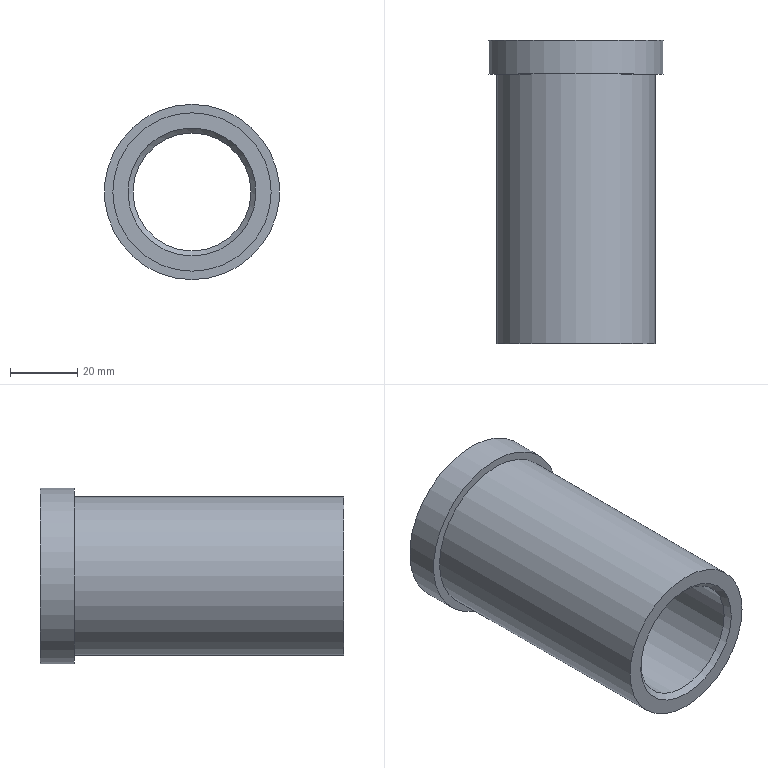Part | STEP file | GUIDE2_id254_x_t | 1 solid | 8 faces | box 52 x 90 x 52 mm | volume 73227 mm3 | cylinder 3 | plane 3 | cone 2 | commonest cylinder face diameters 35 x1 47 x1 52 x1
STEP:
#1=CARTESIAN_POINT('',(-162.,90.5,-216.25));
#2=VERTEX_POINT('',#1);
#3=CARTESIAN_POINT('',(-162.,90.5,-235.));
#4=DIRECTION('',(0.,1.,0.));
#5=DIRECTION('',(0.,0.,1.));
#6=AXIS2_PLACEMENT_3D('',#3,#4,#5);
#7=CIRCLE('',#6,18.75);
#8=EDGE_CURVE('',#2,#2,#7,.T.);
#9=ORIENTED_EDGE('',*,*,#8,.T.);
#10=EDGE_LOOP('',(#9));
#11=FACE_BOUND('',#10,.T.);
#12=CARTESIAN_POINT('',(-162.,89.25,-252.5));
#13=VERTEX_POINT('',#12);
#14=CARTESIAN_POINT('',(-162.,89.25,-235.));
#15=DIRECTION('',(0.,-1.,0.));
#16=DIRECTION('',(0.,0.,-1.));
#17=AXIS2_PLACEMENT_3D('',#14,#15,#16);
#18=CIRCLE('',#17,17.5);
#19=EDGE_CURVE('',#13,#13,#18,.T.);
#20=ORIENTED_EDGE('',*,*,#19,.T.);
#21=EDGE_LOOP('',(#20));
#22=FACE_BOUND('',#21,.T.);
#23=CARTESIAN_POINT('',(-162.,90.5,-235.));
#24=DIRECTION('',(0.,1.,0.));
#25=DIRECTION('',(0.,0.,1.));
#26=AXIS2_PLACEMENT_3D('',#23,#24,#25);
#27=CONICAL_SURFACE('',#26,18.75,45.);
#28=ADVANCED_FACE('',(#11,#22),#27,.F.);
#29=ORIENTED_EDGE('',*,*,#19,.F.);
#30=EDGE_LOOP('',(#29));
#31=FACE_BOUND('',#30,.T.);
#32=CARTESIAN_POINT('',(-179.5,2.,-235.));
#33=VERTEX_POINT('',#32);
#34=CARTESIAN_POINT('',(-162.,2.,-235.));
#35=DIRECTION('',(0.,-1.,0.));
#36=DIRECTION('',(-1.,0.,0.));
#37=AXIS2_PLACEMENT_3D('',#34,#35,#36);
#38=CIRCLE('',#37,17.5);
#39=EDGE_CURVE('',#33,#33,#38,.T.);
#40=ORIENTED_EDGE('',*,*,#39,.T.);
#41=EDGE_LOOP('',(#40));
#42=FACE_BOUND('',#41,.T.);
#43=CARTESIAN_POINT('',(-162.,-4.,-235.));
#44=DIRECTION('',(0.,-1.,0.));
#45=DIRECTION('',(0.,0.,-1.));
#46=AXIS2_PLACEMENT_3D('',#43,#44,#45);
#47=CYLINDRICAL_SURFACE('',#46,17.5);
#48=ADVANCED_FACE('',(#31,#42),#47,.F.);
#49=ORIENTED_EDGE('',*,*,#8,.F.);
#50=EDGE_LOOP('',(#49));
#51=FACE_BOUND('',#50,.T.);
#52=CARTESIAN_POINT('',(-162.,90.5,-261.));
#53=VERTEX_POINT('',#52);
#54=CARTESIAN_POINT('',(-162.,90.5,-235.));
#55=DIRECTION('',(0.,-1.,0.));
#56=DIRECTION('',(0.,0.,-1.));
#57=AXIS2_PLACEMENT_3D('',#54,#55,#56);
#58=CIRCLE('',#57,26.);
#59=EDGE_CURVE('',#53,#53,#58,.T.);
#60=ORIENTED_EDGE('',*,*,#59,.F.);
#61=EDGE_LOOP('',(#60));
#62=FACE_BOUND('',#61,.T.);
#63=CARTESIAN_POINT('',(-162.,90.5,-235.));
#64=DIRECTION('',(0.,-1.,0.));
#65=DIRECTION('',(0.,0.,-1.));
#66=AXIS2_PLACEMENT_3D('',#63,#64,#65);
#67=PLANE('',#66);
#68=ADVANCED_FACE('',(#51,#62),#67,.F.);
#69=ORIENTED_EDGE('',*,*,#39,.F.);
#70=EDGE_LOOP('',(#69));
#71=FACE_BOUND('',#70,.T.);
#72=CARTESIAN_POINT('',(-162.,0.5,-254.));
#73=VERTEX_POINT('',#72);
#74=CARTESIAN_POINT('',(-162.,0.5,-235.));
#75=DIRECTION('',(0.,1.,0.));
#76=DIRECTION('',(0.,0.,-1.));
#77=AXIS2_PLACEMENT_3D('',#74,#75,#76);
#78=CIRCLE('',#77,19.);
#79=EDGE_CURVE('',#73,#73,#78,.T.);
#80=ORIENTED_EDGE('',*,*,#79,.F.);
#81=EDGE_LOOP('',(#80));
#82=FACE_BOUND('',#81,.T.);
#83=CARTESIAN_POINT('',(-162.,0.5,-235.));
#84=DIRECTION('',(0.,-1.,0.));
#85=DIRECTION('',(0.,0.,-1.));
#86=AXIS2_PLACEMENT_3D('',#83,#84,#85);
#87=CONICAL_SURFACE('',#86,19.,45.);
#88=ADVANCED_FACE('',(#71,#82),#87,.F.);
#89=ORIENTED_EDGE('',*,*,#59,.T.);
#90=EDGE_LOOP('',(#89));
#91=FACE_BOUND('',#90,.T.);
#92=CARTESIAN_POINT('',(-162.,80.5,-261.));
#93=VERTEX_POINT('',#92);
#94=CARTESIAN_POINT('',(-162.,80.5,-235.));
#95=DIRECTION('',(0.,-1.,0.));
#96=DIRECTION('',(0.,0.,-1.));
#97=AXIS2_PLACEMENT_3D('',#94,#95,#96);
#98=CIRCLE('',#97,26.);
#99=EDGE_CURVE('',#93,#93,#98,.T.);
#100=ORIENTED_EDGE('',*,*,#99,.F.);
#101=EDGE_LOOP('',(#100));
#102=FACE_BOUND('',#101,.T.);
#103=CARTESIAN_POINT('',(-162.,-4.,-235.));
#104=DIRECTION('',(0.,-1.,0.));
#105=DIRECTION('',(0.,0.,-1.));
#106=AXIS2_PLACEMENT_3D('',#103,#104,#105);
#107=CYLINDRICAL_SURFACE('',#106,26.);
#108=ADVANCED_FACE('',(#91,#102),#107,.T.);
#109=ORIENTED_EDGE('',*,*,#79,.T.);
#110=EDGE_LOOP('',(#109));
#111=FACE_BOUND('',#110,.T.);
#112=CARTESIAN_POINT('',(-162.,0.5,-258.5));
#113=VERTEX_POINT('',#112);
#114=CARTESIAN_POINT('',(-162.,0.5,-235.));
#115=DIRECTION('',(0.,1.,0.));
#116=DIRECTION('',(0.,0.,-1.));
#117=AXIS2_PLACEMENT_3D('',#114,#115,#116);
#118=CIRCLE('',#117,23.5);
#119=EDGE_CURVE('',#113,#113,#118,.T.);
#120=ORIENTED_EDGE('',*,*,#119,.F.);
#121=EDGE_LOOP('',(#120));
#122=FACE_BOUND('',#121,.T.);
#123=CARTESIAN_POINT('',(-162.,0.5,-235.));
#124=DIRECTION('',(0.,-1.,0.));
#125=DIRECTION('',(0.,0.,-1.));
#126=AXIS2_PLACEMENT_3D('',#123,#124,#125);
#127=PLANE('',#126);
#128=ADVANCED_FACE('',(#111,#122),#127,.T.);
#129=CARTESIAN_POINT('',(-162.,80.5,-258.5));
#130=VERTEX_POINT('',#129);
#131=CARTESIAN_POINT('',(-162.,80.5,-235.));
#132=DIRECTION('',(0.,-1.,0.));
#133=DIRECTION('',(0.,0.,-1.));
#134=AXIS2_PLACEMENT_3D('',#131,#132,#133);
#135=CIRCLE('',#134,23.5);
#136=EDGE_CURVE('',#130,#130,#135,.T.);
#137=ORIENTED_EDGE('',*,*,#136,.F.);
#138=EDGE_LOOP('',(#137));
#139=FACE_BOUND('',#138,.T.);
#140=ORIENTED_EDGE('',*,*,#99,.T.);
#141=EDGE_LOOP('',(#140));
#142=FACE_BOUND('',#141,.T.);
#143=CARTESIAN_POINT('',(-162.,80.5,-235.));
#144=DIRECTION('',(0.,-1.,0.));
#145=DIRECTION('',(0.,0.,-1.));
#146=AXIS2_PLACEMENT_3D('',#143,#144,#145);
#147=PLANE('',#146);
#148=ADVANCED_FACE('',(#139,#142),#147,.T.);
#149=ORIENTED_EDGE('',*,*,#136,.T.);
#150=EDGE_LOOP('',(#149));
#151=FACE_BOUND('',#150,.T.);
#152=ORIENTED_EDGE('',*,*,#119,.T.);
#153=EDGE_LOOP('',(#152));
#154=FACE_BOUND('',#153,.T.);
#155=CARTESIAN_POINT('',(-162.,-4.,-235.));
#156=DIRECTION('',(0.,-1.,0.));
#157=DIRECTION('',(0.,0.,-1.));
#158=AXIS2_PLACEMENT_3D('',#155,#156,#157);
#159=CYLINDRICAL_SURFACE('',#158,23.5);
#160=ADVANCED_FACE('',(#151,#154),#159,.T.);
#161=CLOSED_SHELL('',(#28,#48,#68,#88,#108,#128,#148,#160));
#162=MANIFOLD_SOLID_BREP('',#161);
#163=(LENGTH_UNIT()NAMED_UNIT(*)SI_UNIT(.MILLI.,.METRE.));
#164=UNCERTAINTY_MEASURE_WITH_UNIT(LENGTH_MEASURE(0.00002),#163,'','');
#165=(NAMED_UNIT(*)PLANE_ANGLE_UNIT()SI_UNIT($,.RADIAN.));
#166=PLANE_ANGLE_MEASURE_WITH_UNIT(PLANE_ANGLE_MEASURE(0.01745),#165);
#167=DIMENSIONAL_EXPONENTS(0.,0.,0.,0.,0.,0.,0.);
#168=(CONVERSION_BASED_UNIT('DEGREE',#166)NAMED_UNIT(#167)PLANE_ANGLE_UNIT());
#169=(NAMED_UNIT(*)SI_UNIT($,.STERADIAN.)SOLID_ANGLE_UNIT());
#170=(GEOMETRIC_REPRESENTATION_CONTEXT(3)GLOBAL_UNCERTAINTY_ASSIGNED_CONTEXT((#164))GLOBAL_UNIT_ASSIGNED_CONTEXT((#163,#168,#169))REPRESENTATION_CONTEXT('',''));
#171=ADVANCED_BREP_SHAPE_REPRESENTATION('',(#162),#170);